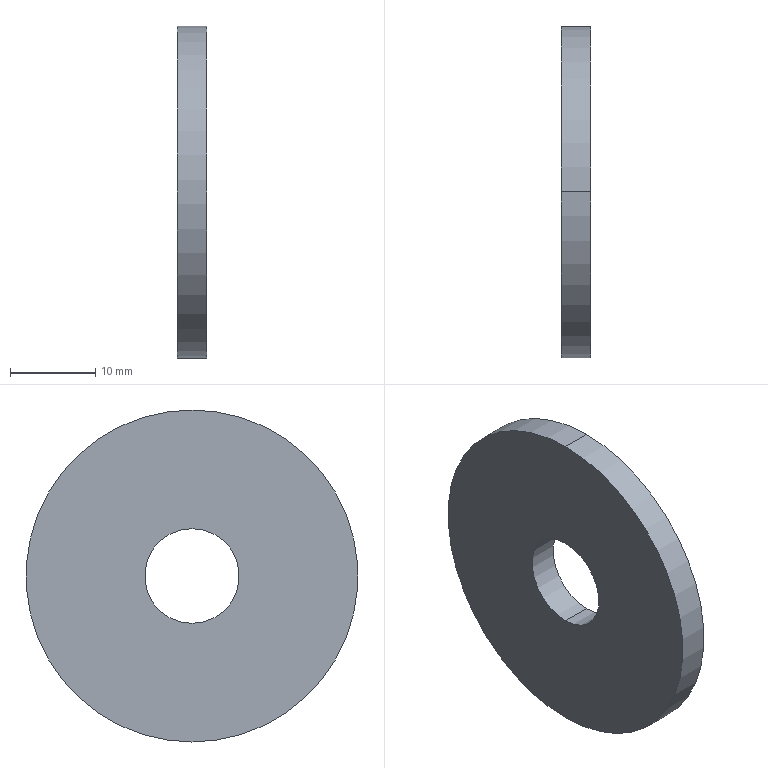Part | STEP file | flat washer wide_am_B18.22M - Plain washer, 10 mm, wide | 1 solid | 6 faces | box 3.5 x 39 x 39 mm | volume 3841 mm3 | cylinder 4 | plane 2 | commonest cylinder face diameters 11.12 x2 39 x2
STEP:
#1=CARTESIAN_POINT('',(0.,0.,0.));
#2=DIRECTION('',(0.,0.,1.));
#3=DIRECTION('',(1.,0.,0.));
#4=AXIS2_PLACEMENT_3D('',#1,#2,#3);
#5=CARTESIAN_POINT('',(0.,0.,19.5));
#6=VERTEX_POINT('',#5);
#7=CARTESIAN_POINT('',(0.,0.,-19.5));
#8=VERTEX_POINT('',#7);
#9=CARTESIAN_POINT('',(0.,0.,0.));
#10=DIRECTION('',(-1.,0.,0.));
#11=DIRECTION('',(0.,0.,1.));
#12=AXIS2_PLACEMENT_3D('',#9,#10,#11);
#13=CIRCLE('',#12,19.5);
#14=CARTESIAN_POINT('',(-34.925,0.,0.));
#15=DIRECTION('',(-1.,0.,0.));
#16=DIRECTION('',(0.,0.,1.));
#17=AXIS2_PLACEMENT_3D('',#14,#15,#16);
#18=CYLINDRICAL_SURFACE('',#17,19.5);
#19=CARTESIAN_POINT('',(0.,-34.925));
#20=DIRECTION('',(1.,0.));
#21=VECTOR('',#20,1.);
#22=LINE('',#19,#21);
#23=(GEOMETRIC_REPRESENTATION_CONTEXT(2)PARAMETRIC_REPRESENTATION_CONTEXT()REPRESENTATION_CONTEXT('',''));
#24=DEFINITIONAL_REPRESENTATION('',(#22),#23);
#25=PCURVE('',#18,#24);
#26=CARTESIAN_POINT('',(0.,5.56,0.));
#27=DIRECTION('',(-1.,0.,0.));
#28=DIRECTION('',(0.,0.,1.));
#29=AXIS2_PLACEMENT_3D('',#26,#27,#28);
#30=PLANE('',#29);
#31=CARTESIAN_POINT('',(0.,-5.56));
#32=DIRECTION('',(1.,0.));
#33=AXIS2_PLACEMENT_2D('',#31,#32);
#34=CIRCLE('',#33,19.5);
#35=(GEOMETRIC_REPRESENTATION_CONTEXT(2)PARAMETRIC_REPRESENTATION_CONTEXT()REPRESENTATION_CONTEXT('',''));
#36=DEFINITIONAL_REPRESENTATION('',(#34),#35);
#37=PCURVE('',#30,#36);
#38=SURFACE_CURVE('',#13,(#25,#37),.PCURVE_S1.);
#39=EDGE_CURVE('',#6,#8,#38,.T.);
#40=ORIENTED_EDGE('',*,*,#39,.T.);
#41=CARTESIAN_POINT('',(-3.5,0.,-19.5));
#42=VERTEX_POINT('',#41);
#43=CARTESIAN_POINT('',(-34.925,0.,-19.5));
#44=DIRECTION('',(-1.,0.,0.));
#45=VECTOR('',#44,1.);
#46=LINE('',#43,#45);
#47=CARTESIAN_POINT('',(3.142,0.));
#48=DIRECTION('',(0.,1.));
#49=VECTOR('',#48,1.);
#50=LINE('',#47,#49);
#51=(GEOMETRIC_REPRESENTATION_CONTEXT(2)PARAMETRIC_REPRESENTATION_CONTEXT()REPRESENTATION_CONTEXT('',''));
#52=DEFINITIONAL_REPRESENTATION('',(#50),#51);
#53=PCURVE('',#18,#52);
#54=CARTESIAN_POINT('',(-34.925,0.,0.));
#55=DIRECTION('',(-1.,0.,0.));
#56=DIRECTION('',(0.,0.,1.));
#57=AXIS2_PLACEMENT_3D('',#54,#55,#56);
#58=CYLINDRICAL_SURFACE('',#57,19.5);
#59=CARTESIAN_POINT('',(3.142,0.));
#60=DIRECTION('',(0.,1.));
#61=VECTOR('',#60,1.);
#62=LINE('',#59,#61);
#63=(GEOMETRIC_REPRESENTATION_CONTEXT(2)PARAMETRIC_REPRESENTATION_CONTEXT()REPRESENTATION_CONTEXT('',''));
#64=DEFINITIONAL_REPRESENTATION('',(#62),#63);
#65=PCURVE('',#58,#64);
#66=SURFACE_CURVE('',#46,(#53,#65),.PCURVE_S1.);
#67=EDGE_CURVE('',#8,#42,#66,.T.);
#68=ORIENTED_EDGE('',*,*,#67,.T.);
#69=CARTESIAN_POINT('',(-3.5,0.,19.5));
#70=VERTEX_POINT('',#69);
#71=CARTESIAN_POINT('',(-3.5,0.,0.));
#72=DIRECTION('',(-1.,0.,0.));
#73=DIRECTION('',(0.,0.,1.));
#74=AXIS2_PLACEMENT_3D('',#71,#72,#73);
#75=CIRCLE('',#74,19.5);
#76=CARTESIAN_POINT('',(0.,-31.425));
#77=DIRECTION('',(1.,0.));
#78=VECTOR('',#77,1.);
#79=LINE('',#76,#78);
#80=(GEOMETRIC_REPRESENTATION_CONTEXT(2)PARAMETRIC_REPRESENTATION_CONTEXT()REPRESENTATION_CONTEXT('',''));
#81=DEFINITIONAL_REPRESENTATION('',(#79),#80);
#82=PCURVE('',#18,#81);
#83=CARTESIAN_POINT('',(-3.5,19.5,0.));
#84=DIRECTION('',(1.,0.,0.));
#85=DIRECTION('',(0.,0.,-1.));
#86=AXIS2_PLACEMENT_3D('',#83,#84,#85);
#87=PLANE('',#86);
#88=CARTESIAN_POINT('',(-19.5,-19.5));
#89=CARTESIAN_POINT('',(-19.5,14.275));
#90=CARTESIAN_POINT('',(9.75,-2.613));
#91=CARTESIAN_POINT('',(39.,-19.5));
#92=CARTESIAN_POINT('',(9.75,-36.387));
#93=CARTESIAN_POINT('',(-19.5,-53.275));
#94=CARTESIAN_POINT('',(-19.5,-19.5));
#95=(BOUNDED_CURVE()B_SPLINE_CURVE(2,(#88,#89,#90,#91,#92,#93,#94),.UNSPECIFIED.,.T.,.F.)B_SPLINE_CURVE_WITH_KNOTS((1,2,2,2,2,1),(-2.094,0.,2.094,4.189,6.283,8.378),.UNSPECIFIED.)CURVE()GEOMETRIC_REPRESENTATION_ITEM()RATIONAL_B_SPLINE_CURVE((1.,0.5,1.,0.5,1.,0.5,1.))REPRESENTATION_ITEM(''));
#96=(GEOMETRIC_REPRESENTATION_CONTEXT(2)PARAMETRIC_REPRESENTATION_CONTEXT()REPRESENTATION_CONTEXT('',''));
#97=DEFINITIONAL_REPRESENTATION('',(#95),#96);
#98=PCURVE('',#87,#97);
#99=SURFACE_CURVE('',#75,(#82,#98),.PCURVE_S1.);
#100=EDGE_CURVE('',#70,#42,#99,.T.);
#101=ORIENTED_EDGE('',*,*,#100,.F.);
#102=CARTESIAN_POINT('',(-34.925,0.,19.5));
#103=DIRECTION('',(-1.,0.,0.));
#104=VECTOR('',#103,1.);
#105=LINE('',#102,#104);
#106=CARTESIAN_POINT('',(0.,0.));
#107=DIRECTION('',(0.,1.));
#108=VECTOR('',#107,1.);
#109=LINE('',#106,#108);
#110=(GEOMETRIC_REPRESENTATION_CONTEXT(2)PARAMETRIC_REPRESENTATION_CONTEXT()REPRESENTATION_CONTEXT('',''));
#111=DEFINITIONAL_REPRESENTATION('',(#109),#110);
#112=PCURVE('',#18,#111);
#113=CARTESIAN_POINT('',(6.283,0.));
#114=DIRECTION('',(0.,1.));
#115=VECTOR('',#114,1.);
#116=LINE('',#113,#115);
#117=(GEOMETRIC_REPRESENTATION_CONTEXT(2)PARAMETRIC_REPRESENTATION_CONTEXT()REPRESENTATION_CONTEXT('',''));
#118=DEFINITIONAL_REPRESENTATION('',(#116),#117);
#119=PCURVE('',#58,#118);
#120=SURFACE_CURVE('',#105,(#112,#119),.PCURVE_S1.);
#121=EDGE_CURVE('',#6,#70,#120,.T.);
#122=ORIENTED_EDGE('',*,*,#121,.F.);
#123=EDGE_LOOP('',(#40,#68,#101,#122));
#124=FACE_BOUND('',#123,.T.);
#125=ADVANCED_FACE('',(#124),#18,.T.);
#126=CARTESIAN_POINT('',(0.,0.,5.56));
#127=VERTEX_POINT('',#126);
#128=CARTESIAN_POINT('',(-3.5,0.,5.56));
#129=VERTEX_POINT('',#128);
#130=CARTESIAN_POINT('',(-34.925,0.,5.56));
#131=DIRECTION('',(-1.,0.,0.));
#132=VECTOR('',#131,1.);
#133=LINE('',#130,#132);
#134=CARTESIAN_POINT('',(-34.925,0.,0.));
#135=DIRECTION('',(-1.,0.,0.));
#136=DIRECTION('',(0.,0.,1.));
#137=AXIS2_PLACEMENT_3D('',#134,#135,#136);
#138=CYLINDRICAL_SURFACE('',#137,5.56);
#139=CARTESIAN_POINT('',(6.283,0.));
#140=DIRECTION('',(0.,1.));
#141=VECTOR('',#140,1.);
#142=LINE('',#139,#141);
#143=(GEOMETRIC_REPRESENTATION_CONTEXT(2)PARAMETRIC_REPRESENTATION_CONTEXT()REPRESENTATION_CONTEXT('',''));
#144=DEFINITIONAL_REPRESENTATION('',(#142),#143);
#145=PCURVE('',#138,#144);
#146=CARTESIAN_POINT('',(-34.925,0.,0.));
#147=DIRECTION('',(-1.,0.,0.));
#148=DIRECTION('',(0.,0.,1.));
#149=AXIS2_PLACEMENT_3D('',#146,#147,#148);
#150=CYLINDRICAL_SURFACE('',#149,5.56);
#151=CARTESIAN_POINT('',(0.,0.));
#152=DIRECTION('',(0.,1.));
#153=VECTOR('',#152,1.);
#154=LINE('',#151,#153);
#155=(GEOMETRIC_REPRESENTATION_CONTEXT(2)PARAMETRIC_REPRESENTATION_CONTEXT()REPRESENTATION_CONTEXT('',''));
#156=DEFINITIONAL_REPRESENTATION('',(#154),#155);
#157=PCURVE('',#150,#156);
#158=SURFACE_CURVE('',#133,(#145,#157),.PCURVE_S1.);
#159=EDGE_CURVE('',#127,#129,#158,.T.);
#160=ORIENTED_EDGE('',*,*,#159,.T.);
#161=CARTESIAN_POINT('',(-3.5,0.,-5.56));
#162=VERTEX_POINT('',#161);
#163=CARTESIAN_POINT('',(-3.5,0.,0.));
#164=DIRECTION('',(-1.,0.,0.));
#165=DIRECTION('',(0.,0.,1.));
#166=AXIS2_PLACEMENT_3D('',#163,#164,#165);
#167=CIRCLE('',#166,5.56);
#168=CARTESIAN_POINT('',(0.,-31.425));
#169=DIRECTION('',(1.,0.));
#170=VECTOR('',#169,1.);
#171=LINE('',#168,#170);
#172=(GEOMETRIC_REPRESENTATION_CONTEXT(2)PARAMETRIC_REPRESENTATION_CONTEXT()REPRESENTATION_CONTEXT('',''));
#173=DEFINITIONAL_REPRESENTATION('',(#171),#172);
#174=PCURVE('',#138,#173);
#175=CARTESIAN_POINT('',(-5.56,-19.5));
#176=CARTESIAN_POINT('',(-5.56,-9.87));
#177=CARTESIAN_POINT('',(2.78,-14.685));
#178=CARTESIAN_POINT('',(11.12,-19.5));
#179=CARTESIAN_POINT('',(2.78,-24.315));
#180=CARTESIAN_POINT('',(-5.56,-29.13));
#181=CARTESIAN_POINT('',(-5.56,-19.5));
#182=(BOUNDED_CURVE()B_SPLINE_CURVE(2,(#175,#176,#177,#178,#179,#180,#181),.UNSPECIFIED.,.T.,.F.)B_SPLINE_CURVE_WITH_KNOTS((1,2,2,2,2,1),(-2.094,0.,2.094,4.189,6.283,8.378),.UNSPECIFIED.)CURVE()GEOMETRIC_REPRESENTATION_ITEM()RATIONAL_B_SPLINE_CURVE((1.,0.5,1.,0.5,1.,0.5,1.))REPRESENTATION_ITEM(''));
#183=(GEOMETRIC_REPRESENTATION_CONTEXT(2)PARAMETRIC_REPRESENTATION_CONTEXT()REPRESENTATION_CONTEXT('',''));
#184=DEFINITIONAL_REPRESENTATION('',(#182),#183);
#185=PCURVE('',#87,#184);
#186=SURFACE_CURVE('',#167,(#174,#185),.PCURVE_S1.);
#187=EDGE_CURVE('',#162,#129,#186,.T.);
#188=ORIENTED_EDGE('',*,*,#187,.F.);
#189=CARTESIAN_POINT('',(0.,0.,-5.56));
#190=VERTEX_POINT('',#189);
#191=CARTESIAN_POINT('',(-34.925,0.,-5.56));
#192=DIRECTION('',(-1.,0.,0.));
#193=VECTOR('',#192,1.);
#194=LINE('',#191,#193);
#195=CARTESIAN_POINT('',(3.142,0.));
#196=DIRECTION('',(0.,1.));
#197=VECTOR('',#196,1.);
#198=LINE('',#195,#197);
#199=(GEOMETRIC_REPRESENTATION_CONTEXT(2)PARAMETRIC_REPRESENTATION_CONTEXT()REPRESENTATION_CONTEXT('',''));
#200=DEFINITIONAL_REPRESENTATION('',(#198),#199);
#201=PCURVE('',#138,#200);
#202=CARTESIAN_POINT('',(3.142,0.));
#203=DIRECTION('',(0.,1.));
#204=VECTOR('',#203,1.);
#205=LINE('',#202,#204);
#206=(GEOMETRIC_REPRESENTATION_CONTEXT(2)PARAMETRIC_REPRESENTATION_CONTEXT()REPRESENTATION_CONTEXT('',''));
#207=DEFINITIONAL_REPRESENTATION('',(#205),#206);
#208=PCURVE('',#150,#207);
#209=SURFACE_CURVE('',#194,(#201,#208),.PCURVE_S1.);
#210=EDGE_CURVE('',#190,#162,#209,.T.);
#211=ORIENTED_EDGE('',*,*,#210,.F.);
#212=CARTESIAN_POINT('',(0.,0.,0.));
#213=DIRECTION('',(-1.,0.,0.));
#214=DIRECTION('',(0.,0.,1.));
#215=AXIS2_PLACEMENT_3D('',#212,#213,#214);
#216=CIRCLE('',#215,5.56);
#217=CARTESIAN_POINT('',(0.,-34.925));
#218=DIRECTION('',(1.,0.));
#219=VECTOR('',#218,1.);
#220=LINE('',#217,#219);
#221=(GEOMETRIC_REPRESENTATION_CONTEXT(2)PARAMETRIC_REPRESENTATION_CONTEXT()REPRESENTATION_CONTEXT('',''));
#222=DEFINITIONAL_REPRESENTATION('',(#220),#221);
#223=PCURVE('',#138,#222);
#224=CARTESIAN_POINT('',(0.,-5.56));
#225=DIRECTION('',(1.,0.));
#226=AXIS2_PLACEMENT_2D('',#224,#225);
#227=CIRCLE('',#226,5.56);
#228=(GEOMETRIC_REPRESENTATION_CONTEXT(2)PARAMETRIC_REPRESENTATION_CONTEXT()REPRESENTATION_CONTEXT('',''));
#229=DEFINITIONAL_REPRESENTATION('',(#227),#228);
#230=PCURVE('',#30,#229);
#231=SURFACE_CURVE('',#216,(#223,#230),.PCURVE_S1.);
#232=EDGE_CURVE('',#190,#127,#231,.T.);
#233=ORIENTED_EDGE('',*,*,#232,.T.);
#234=EDGE_LOOP('',(#160,#188,#211,#233));
#235=FACE_BOUND('',#234,.F.);
#236=ADVANCED_FACE('',(#235),#138,.F.);
#237=CARTESIAN_POINT('',(-3.5,0.,0.));
#238=DIRECTION('',(-1.,0.,0.));
#239=DIRECTION('',(0.,0.,1.));
#240=AXIS2_PLACEMENT_3D('',#237,#238,#239);
#241=CIRCLE('',#240,5.56);
#242=CARTESIAN_POINT('',(0.,-31.425));
#243=DIRECTION('',(1.,0.));
#244=VECTOR('',#243,1.);
#245=LINE('',#242,#244);
#246=(GEOMETRIC_REPRESENTATION_CONTEXT(2)PARAMETRIC_REPRESENTATION_CONTEXT()REPRESENTATION_CONTEXT('',''));
#247=DEFINITIONAL_REPRESENTATION('',(#245),#246);
#248=PCURVE('',#150,#247);
#249=CARTESIAN_POINT('',(-5.56,-19.5));
#250=CARTESIAN_POINT('',(-5.56,-9.87));
#251=CARTESIAN_POINT('',(2.78,-14.685));
#252=CARTESIAN_POINT('',(11.12,-19.5));
#253=CARTESIAN_POINT('',(2.78,-24.315));
#254=CARTESIAN_POINT('',(-5.56,-29.13));
#255=CARTESIAN_POINT('',(-5.56,-19.5));
#256=(BOUNDED_CURVE()B_SPLINE_CURVE(2,(#249,#250,#251,#252,#253,#254,#255),.UNSPECIFIED.,.T.,.F.)B_SPLINE_CURVE_WITH_KNOTS((1,2,2,2,2,1),(-2.094,0.,2.094,4.189,6.283,8.378),.UNSPECIFIED.)CURVE()GEOMETRIC_REPRESENTATION_ITEM()RATIONAL_B_SPLINE_CURVE((1.,0.5,1.,0.5,1.,0.5,1.))REPRESENTATION_ITEM(''));
#257=(GEOMETRIC_REPRESENTATION_CONTEXT(2)PARAMETRIC_REPRESENTATION_CONTEXT()REPRESENTATION_CONTEXT('',''));
#258=DEFINITIONAL_REPRESENTATION('',(#256),#257);
#259=PCURVE('',#87,#258);
#260=SURFACE_CURVE('',#241,(#248,#259),.PCURVE_S1.);
#261=EDGE_CURVE('',#129,#162,#260,.T.);
#262=ORIENTED_EDGE('',*,*,#261,.F.);
#263=ORIENTED_EDGE('',*,*,#159,.F.);
#264=CARTESIAN_POINT('',(0.,0.,0.));
#265=DIRECTION('',(-1.,0.,0.));
#266=DIRECTION('',(0.,0.,1.));
#267=AXIS2_PLACEMENT_3D('',#264,#265,#266);
#268=CIRCLE('',#267,5.56);
#269=CARTESIAN_POINT('',(0.,-34.925));
#270=DIRECTION('',(1.,0.));
#271=VECTOR('',#270,1.);
#272=LINE('',#269,#271);
#273=(GEOMETRIC_REPRESENTATION_CONTEXT(2)PARAMETRIC_REPRESENTATION_CONTEXT()REPRESENTATION_CONTEXT('',''));
#274=DEFINITIONAL_REPRESENTATION('',(#272),#273);
#275=PCURVE('',#150,#274);
#276=CARTESIAN_POINT('',(0.,-5.56));
#277=DIRECTION('',(1.,0.));
#278=AXIS2_PLACEMENT_2D('',#276,#277);
#279=CIRCLE('',#278,5.56);
#280=(GEOMETRIC_REPRESENTATION_CONTEXT(2)PARAMETRIC_REPRESENTATION_CONTEXT()REPRESENTATION_CONTEXT('',''));
#281=DEFINITIONAL_REPRESENTATION('',(#279),#280);
#282=PCURVE('',#30,#281);
#283=SURFACE_CURVE('',#268,(#275,#282),.PCURVE_S1.);
#284=EDGE_CURVE('',#127,#190,#283,.T.);
#285=ORIENTED_EDGE('',*,*,#284,.T.);
#286=ORIENTED_EDGE('',*,*,#210,.T.);
#287=EDGE_LOOP('',(#262,#263,#285,#286));
#288=FACE_BOUND('',#287,.F.);
#289=ADVANCED_FACE('',(#288),#150,.F.);
#290=ORIENTED_EDGE('',*,*,#39,.F.);
#291=CARTESIAN_POINT('',(0.,0.,0.));
#292=DIRECTION('',(-1.,0.,0.));
#293=DIRECTION('',(0.,0.,1.));
#294=AXIS2_PLACEMENT_3D('',#291,#292,#293);
#295=CIRCLE('',#294,19.5);
#296=CARTESIAN_POINT('',(0.,-5.56));
#297=DIRECTION('',(1.,0.));
#298=AXIS2_PLACEMENT_2D('',#296,#297);
#299=CIRCLE('',#298,19.5);
#300=(GEOMETRIC_REPRESENTATION_CONTEXT(2)PARAMETRIC_REPRESENTATION_CONTEXT()REPRESENTATION_CONTEXT('',''));
#301=DEFINITIONAL_REPRESENTATION('',(#299),#300);
#302=PCURVE('',#30,#301);
#303=CARTESIAN_POINT('',(0.,-34.925));
#304=DIRECTION('',(1.,0.));
#305=VECTOR('',#304,1.);
#306=LINE('',#303,#305);
#307=(GEOMETRIC_REPRESENTATION_CONTEXT(2)PARAMETRIC_REPRESENTATION_CONTEXT()REPRESENTATION_CONTEXT('',''));
#308=DEFINITIONAL_REPRESENTATION('',(#306),#307);
#309=PCURVE('',#58,#308);
#310=SURFACE_CURVE('',#295,(#302,#309),.PCURVE_S1.);
#311=EDGE_CURVE('',#8,#6,#310,.T.);
#312=ORIENTED_EDGE('',*,*,#311,.F.);
#313=EDGE_LOOP('',(#290,#312));
#314=FACE_BOUND('',#313,.T.);
#315=ORIENTED_EDGE('',*,*,#284,.T.);
#316=ORIENTED_EDGE('',*,*,#232,.T.);
#317=EDGE_LOOP('',(#315,#316));
#318=FACE_BOUND('',#317,.T.);
#319=ADVANCED_FACE('',(#314,#318),#30,.F.);
#320=ORIENTED_EDGE('',*,*,#67,.F.);
#321=ORIENTED_EDGE('',*,*,#311,.T.);
#322=ORIENTED_EDGE('',*,*,#121,.T.);
#323=CARTESIAN_POINT('',(-3.5,0.,0.));
#324=DIRECTION('',(-1.,0.,0.));
#325=DIRECTION('',(0.,0.,1.));
#326=AXIS2_PLACEMENT_3D('',#323,#324,#325);
#327=CIRCLE('',#326,19.5);
#328=CARTESIAN_POINT('',(0.,-31.425));
#329=DIRECTION('',(1.,0.));
#330=VECTOR('',#329,1.);
#331=LINE('',#328,#330);
#332=(GEOMETRIC_REPRESENTATION_CONTEXT(2)PARAMETRIC_REPRESENTATION_CONTEXT()REPRESENTATION_CONTEXT('',''));
#333=DEFINITIONAL_REPRESENTATION('',(#331),#332);
#334=PCURVE('',#58,#333);
#335=CARTESIAN_POINT('',(-19.5,-19.5));
#336=CARTESIAN_POINT('',(-19.5,14.275));
#337=CARTESIAN_POINT('',(9.75,-2.613));
#338=CARTESIAN_POINT('',(39.,-19.5));
#339=CARTESIAN_POINT('',(9.75,-36.387));
#340=CARTESIAN_POINT('',(-19.5,-53.275));
#341=CARTESIAN_POINT('',(-19.5,-19.5));
#342=(BOUNDED_CURVE()B_SPLINE_CURVE(2,(#335,#336,#337,#338,#339,#340,#341),.UNSPECIFIED.,.T.,.F.)B_SPLINE_CURVE_WITH_KNOTS((1,2,2,2,2,1),(-2.094,0.,2.094,4.189,6.283,8.378),.UNSPECIFIED.)CURVE()GEOMETRIC_REPRESENTATION_ITEM()RATIONAL_B_SPLINE_CURVE((1.,0.5,1.,0.5,1.,0.5,1.))REPRESENTATION_ITEM(''));
#343=(GEOMETRIC_REPRESENTATION_CONTEXT(2)PARAMETRIC_REPRESENTATION_CONTEXT()REPRESENTATION_CONTEXT('',''));
#344=DEFINITIONAL_REPRESENTATION('',(#342),#343);
#345=PCURVE('',#87,#344);
#346=SURFACE_CURVE('',#327,(#334,#345),.PCURVE_S1.);
#347=EDGE_CURVE('',#42,#70,#346,.T.);
#348=ORIENTED_EDGE('',*,*,#347,.F.);
#349=EDGE_LOOP('',(#320,#321,#322,#348));
#350=FACE_BOUND('',#349,.T.);
#351=ADVANCED_FACE('',(#350),#58,.T.);
#352=ORIENTED_EDGE('',*,*,#261,.F.);
#353=ORIENTED_EDGE('',*,*,#187,.F.);
#354=EDGE_LOOP('',(#352,#353));
#355=FACE_BOUND('',#354,.T.);
#356=ORIENTED_EDGE('',*,*,#100,.T.);
#357=ORIENTED_EDGE('',*,*,#347,.T.);
#358=EDGE_LOOP('',(#356,#357));
#359=FACE_BOUND('',#358,.T.);
#360=ADVANCED_FACE('',(#355,#359),#87,.F.);
#361=CLOSED_SHELL('',(#125,#236,#289,#319,#351,#360));
#362=MANIFOLD_SOLID_BREP('',#361);
#363=(LENGTH_UNIT()NAMED_UNIT(*)SI_UNIT(.MILLI.,.METRE.));
#364=UNCERTAINTY_MEASURE_WITH_UNIT(LENGTH_MEASURE(0.0000001),#363,'','');
#365=(NAMED_UNIT(*)PLANE_ANGLE_UNIT()SI_UNIT($,.RADIAN.));
#366=(NAMED_UNIT(*)SI_UNIT($,.STERADIAN.)SOLID_ANGLE_UNIT());
#367=(GEOMETRIC_REPRESENTATION_CONTEXT(3)GLOBAL_UNCERTAINTY_ASSIGNED_CONTEXT((#364))GLOBAL_UNIT_ASSIGNED_CONTEXT((#363,#365,#366))REPRESENTATION_CONTEXT('',''));
#368=ADVANCED_BREP_SHAPE_REPRESENTATION('',(#4,#362),#367);